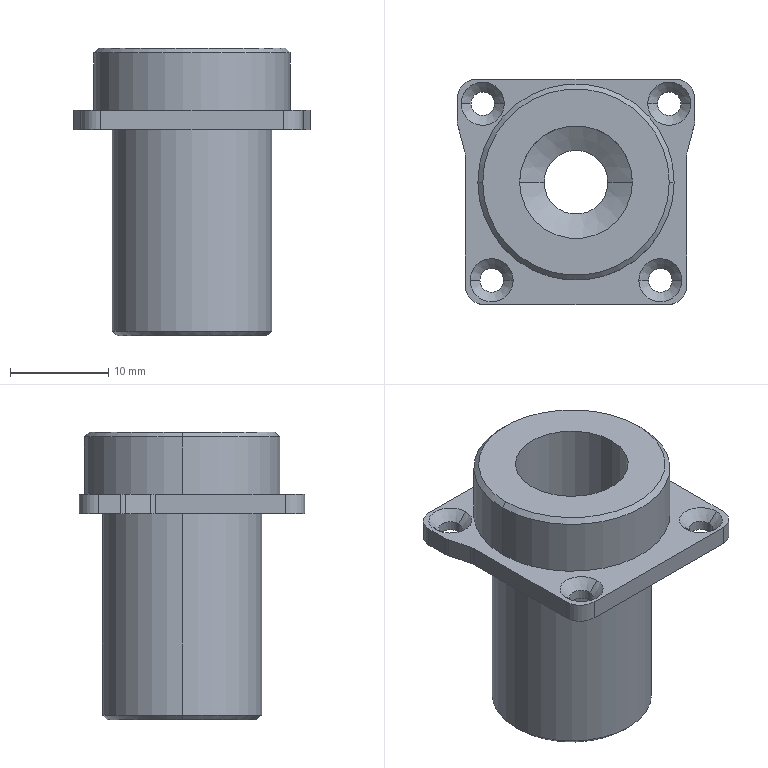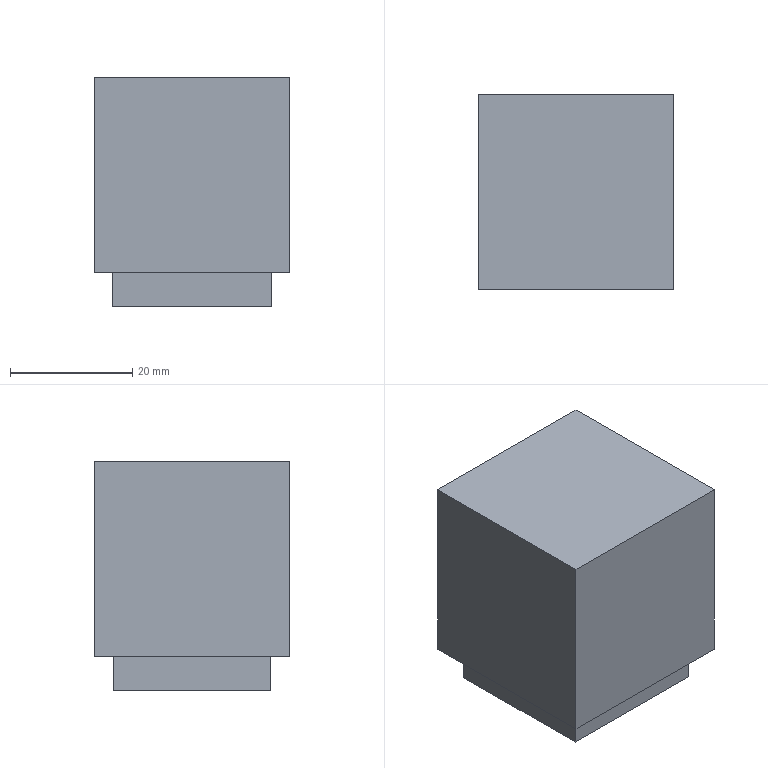CAM job | NX | 3-axis milling, drilling | part box 24.2 x 23 x 29.342 mm | stock box 32 x 32 x 37.658 mm
Tools:
number,name,description,diameter,corner_radius,flute_length,length,flutes
9,螺纹刀D10-T10,Thread Mill,10.0,0.0,20.0,50.0,2
4,D4-12-D4-50-3T-ROUGH,D4-12-D4-50-3T-粗,4.0,0.0,12.0,50.0,2
0,D4-12-D4-50-3T-FINISH,D4-12-D4-50-3T,4.0,0.0,12.0,50.0,3
2,D8-25-D8-60-3T-ROUGH,D8-25-D8-60-3T-粗,8.0,0.0,25.0,60.0,2
3,D8-25-D8-60-3T-FINISH,D8-25-D8-60-3T,8.0,0.0,25.0,60.0,3
1,D50面刀,D50面刀,50.0,0.0,30.0,30.0,4
8,钻头D2.5-35-61,钻刀D2.5-35-61,2.5,0.0,36.0,61.0,2
6,钻头D6.5-73-105,钻刀D6.5-73-105,6.5,0.0,73.0,105.0,2
5,倒角D4-90度,倒角D4-90度,4.0,0.0,5.0,50.0,2
7,D7.9,Milling Tool-5 Parameters,7.9,0.0,30.0,30.0,4
Operations:
program,operation,operation_type,tool,method,geometry_group,spindle_rpm,surface_speed,feed_per_tooth,feed_cut,feed_plunge,cut_length_mm,path_length_mm,cut_time_min,machine_time_min
A1,PLANAR_MILL,PlanarMilling,D50面刀,METHOD,WORKPIECE_54,4500.0,706.0,0.0333,600.0,100.0,84.2,120.2,0.1403,0.1439
A1,动态粗,CavityMilling,D8-25-D8-60-3T-ROUGH,METHOD,WORKPIECE_54,6500.0,100.0,0.1178,3000.0,100.0,740.265,820.965,0.2344,0.2424
A1,DRILLING,Operation,倒角D4-90度,METHOD,WORKPIECE_54,2000.0,25.0,0.05,200.0,0.0,4.0,48.0,0.02,0.0244
A1,DRILLING_COPY,Operation,钻头D6.5-73-105,METHOD,WORKPIECE_54,2000.0,40.0,0.05,200.0,0.0,35.0,110.0,0.175,0.1825
A1,动态粗_1,CavityMilling,D4-12-D4-50-3T-ROUGH,METHOD,WORKPIECE_54,5500.0,69.0,0.1364,1500.0,100.0,261.346,319.846,0.1742,0.1801
A1,动态粗_1_COPY,CavityMilling,D4-12-D4-50-3T-ROUGH,METHOD,WORKPIECE_54,5500.0,69.0,0.1364,1500.0,100.0,209.661,617.065,0.1398,0.1805
A1,PLANAR_MILL_1,PlanarMilling,D8-25-D8-60-3T-FINISH,METHOD,WORKPIECE_54,4500.0,113.0,0.0444,600.0,100.0,199.741,277.741,0.3329,0.3407
A1,PLANAR_MILL_1_COPY,PlanarMilling,D8-25-D8-60-3T-FINISH,METHOD,WORKPIECE_54,4500.0,113.0,0.0444,600.0,100.0,87.467,165.467,0.1458,0.1536
A1,DRILLING_1,Operation,D7.9,METHOD,WORKPIECE_54,3500.0,86.0,0.0429,600.0,0.0,3.0,77.5,0.005,0.0125
A1,PLANAR_MILL_7,PlanarMilling,D4-12-D4-50-3T-FINISH,METHOD,A-G54,5500.0,69.0,0.0364,600.0,100.0,75.216,131.017,0.1254,0.1309
A1,平面铣倒角,PlanarMilling,倒角D4-90度,METHOD,WORKPIECE_54,6500.0,100.0,0.1178,1200.0,100.0,65.476,104.476,0.0546,0.0585
B1,动态粗_2,CavityMilling,D8-25-D8-60-3T-ROUGH,METHOD,WORKPIECE_55,6500.0,100.0,0.1178,3000.0,100.0,2205.827,2452.034,0.7124,0.7371
B2,PLANAR_MILL_3_COPY,PlanarMilling,D8-25-D8-60-3T-FINISH,METHOD,WORKPIECE_55,5500.0,138.0,0.0485,800.0,100.0,70.969,106.869,0.0887,0.0923
B2,PLANAR_MILL_3_COPY_COPY,PlanarMilling,D8-25-D8-60-3T-FINISH,METHOD,WORKPIECE_55,5500.0,138.0,0.0485,800.0,100.0,70.969,106.969,0.0887,0.0923
B2,PLANAR_MILL_3,PlanarMilling,D8-25-D8-60-3T-FINISH,METHOD,WORKPIECE_55,5000.0,125.0,0.0333,500.0,100.0,196.496,245.18,0.393,0.3979
B2,PLANAR_MILL_2,PlanarMilling,D8-25-D8-60-3T-FINISH,METHOD,WORKPIECE_55,5500.0,138.0,0.0303,500.0,100.0,242.397,295.281,0.4848,0.4901
B3,PLANAR_MILL_4,PlanarMilling,D4-12-D4-50-3T-ROUGH,METHOD,WORKPIECE_55,6500.0,81.0,0.1154,1500.0,100.0,1400.306,1449.306,0.9335,0.9384
B3,ZLEVEL_PROFILE_STEEP,ZLevelMilling,D4-12-D4-50-3T-ROUGH,METHOD,WORKPIECE_55,5500.0,69.0,0.1818,2000.0,100.0,486.269,548,0.2431,0.2493
B4,DRILLING_2,Operation,倒角D4-90度,METHOD,WORKPIECE_55,3000.0,37.0,0.0333,200.0,0.0,17.2,151.049,0.086,0.0994
B4,PLANAR_MILL_5,PlanarMilling,倒角D4-90度,METHOD,WORKPIECE_55,4500.0,56.0,0.0889,800.0,100.0,73.183,112.183,0.0915,0.0954
B4,PLANAR_MILL_5_COPY,PlanarMilling,倒角D4-90度,METHOD,WORKPIECE_55,4500.0,56.0,0.0889,800.0,100.0,152.094,191.094,0.1901,0.194
B4,PLANAR_MILL_6,PlanarMilling,倒角D4-90度,METHOD,WORKPIECE_55,4500.0,56.0,0.1111,1000.0,100.0,108.644,161.129,0.1086,0.1139
B5,DRILLING_3,Operation,钻头D2.5-35-61,METHOD,WORKPIECE_55,3000.0,23.0,0.0333,200.0,0.0,28.0,172.649,0.14,0.1545
B6,THREAD_MILLING,ThreadMilling,螺纹刀D10-T10,METHOD,WORKPIECE_55,5500.0,172.0,0.0364,400.0,100.0,123.292,197.224,0.3082,0.3156